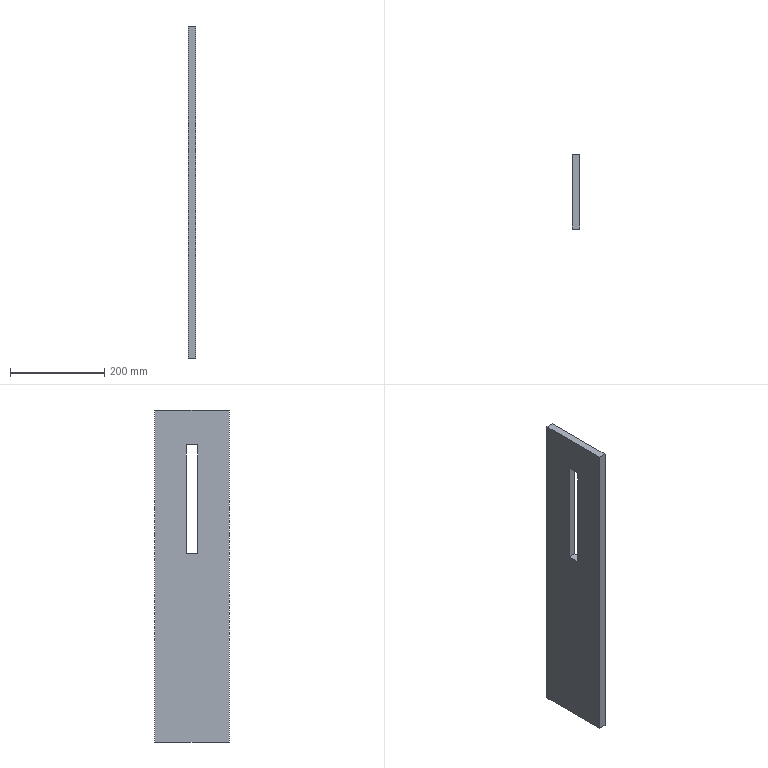Part | STEP file | 05-Vertical plate 1 | 1 solid | 10 faces | box 16 x 158 x 703 mm | volume 1685184 mm3 | plane 10
STEP:
#1=CARTESIAN_POINT('',(0.,0.,0.));
#2=DIRECTION('',(0.,0.,1.));
#3=DIRECTION('',(1.,0.,0.));
#4=AXIS2_PLACEMENT_3D('',#1,#2,#3);
#5=CARTESIAN_POINT('',(0.,-91.5,629.));
#6=VERTEX_POINT('',#5);
#7=CARTESIAN_POINT('',(0.,-66.5,629.));
#8=VERTEX_POINT('',#7);
#9=CARTESIAN_POINT('',(0.,-91.5,629.));
#10=DIRECTION('',(0.,1.,0.));
#11=VECTOR('',#10,1.);
#12=LINE('',#9,#11);
#13=CARTESIAN_POINT('',(0.,0.,703.));
#14=DIRECTION('',(1.,0.,0.));
#15=DIRECTION('',(0.,1.,0.));
#16=AXIS2_PLACEMENT_3D('',#13,#14,#15);
#17=PLANE('',#16);
#18=CARTESIAN_POINT('',(-91.5,-74.));
#19=DIRECTION('',(1.,0.));
#20=VECTOR('',#19,1.);
#21=LINE('',#18,#20);
#22=(GEOMETRIC_REPRESENTATION_CONTEXT(2)PARAMETRIC_REPRESENTATION_CONTEXT()REPRESENTATION_CONTEXT('',''));
#23=DEFINITIONAL_REPRESENTATION('',(#21),#22);
#24=PCURVE('',#17,#23);
#25=CARTESIAN_POINT('',(342.,-91.5,629.));
#26=DIRECTION('',(0.,0.,1.));
#27=DIRECTION('',(0.,-1.,0.));
#28=AXIS2_PLACEMENT_3D('',#25,#26,#27);
#29=PLANE('',#28);
#30=CARTESIAN_POINT('',(0.,-342.));
#31=DIRECTION('',(-1.,0.));
#32=VECTOR('',#31,1.);
#33=LINE('',#30,#32);
#34=(GEOMETRIC_REPRESENTATION_CONTEXT(2)PARAMETRIC_REPRESENTATION_CONTEXT()REPRESENTATION_CONTEXT('',''));
#35=DEFINITIONAL_REPRESENTATION('',(#33),#34);
#36=PCURVE('',#29,#35);
#37=SURFACE_CURVE('',#12,(#24,#36),.PCURVE_S1.);
#38=EDGE_CURVE('',#6,#8,#37,.T.);
#39=ORIENTED_EDGE('',*,*,#38,.F.);
#40=CARTESIAN_POINT('',(0.,-91.5,399.));
#41=VERTEX_POINT('',#40);
#42=CARTESIAN_POINT('',(0.,-91.5,399.));
#43=DIRECTION('',(0.,0.,1.));
#44=VECTOR('',#43,1.);
#45=LINE('',#42,#44);
#46=CARTESIAN_POINT('',(-91.5,-304.));
#47=DIRECTION('',(0.,1.));
#48=VECTOR('',#47,1.);
#49=LINE('',#46,#48);
#50=(GEOMETRIC_REPRESENTATION_CONTEXT(2)PARAMETRIC_REPRESENTATION_CONTEXT()REPRESENTATION_CONTEXT('',''));
#51=DEFINITIONAL_REPRESENTATION('',(#49),#50);
#52=PCURVE('',#17,#51);
#53=CARTESIAN_POINT('',(342.,-91.5,399.));
#54=DIRECTION('',(0.,-1.,0.));
#55=DIRECTION('',(-1.,0.,0.));
#56=AXIS2_PLACEMENT_3D('',#53,#54,#55);
#57=PLANE('',#56);
#58=CARTESIAN_POINT('',(342.,0.));
#59=DIRECTION('',(0.,-1.));
#60=VECTOR('',#59,1.);
#61=LINE('',#58,#60);
#62=(GEOMETRIC_REPRESENTATION_CONTEXT(2)PARAMETRIC_REPRESENTATION_CONTEXT()REPRESENTATION_CONTEXT('',''));
#63=DEFINITIONAL_REPRESENTATION('',(#61),#62);
#64=PCURVE('',#57,#63);
#65=SURFACE_CURVE('',#45,(#52,#64),.PCURVE_S1.);
#66=EDGE_CURVE('',#41,#6,#65,.T.);
#67=ORIENTED_EDGE('',*,*,#66,.F.);
#68=CARTESIAN_POINT('',(0.,-66.5,399.));
#69=VERTEX_POINT('',#68);
#70=CARTESIAN_POINT('',(0.,-91.5,399.));
#71=DIRECTION('',(0.,-1.,0.));
#72=VECTOR('',#71,1.);
#73=LINE('',#70,#72);
#74=CARTESIAN_POINT('',(-91.5,-304.));
#75=DIRECTION('',(-1.,0.));
#76=VECTOR('',#75,1.);
#77=LINE('',#74,#76);
#78=(GEOMETRIC_REPRESENTATION_CONTEXT(2)PARAMETRIC_REPRESENTATION_CONTEXT()REPRESENTATION_CONTEXT('',''));
#79=DEFINITIONAL_REPRESENTATION('',(#77),#78);
#80=PCURVE('',#17,#79);
#81=CARTESIAN_POINT('',(342.,-91.5,399.));
#82=DIRECTION('',(0.,0.,-1.));
#83=DIRECTION('',(0.,1.,0.));
#84=AXIS2_PLACEMENT_3D('',#81,#82,#83);
#85=PLANE('',#84);
#86=CARTESIAN_POINT('',(0.,-342.));
#87=DIRECTION('',(-1.,0.));
#88=VECTOR('',#87,1.);
#89=LINE('',#86,#88);
#90=(GEOMETRIC_REPRESENTATION_CONTEXT(2)PARAMETRIC_REPRESENTATION_CONTEXT()REPRESENTATION_CONTEXT('',''));
#91=DEFINITIONAL_REPRESENTATION('',(#89),#90);
#92=PCURVE('',#85,#91);
#93=SURFACE_CURVE('',#73,(#80,#92),.PCURVE_S1.);
#94=EDGE_CURVE('',#69,#41,#93,.T.);
#95=ORIENTED_EDGE('',*,*,#94,.F.);
#96=CARTESIAN_POINT('',(0.,-66.5,399.));
#97=DIRECTION('',(0.,0.,-1.));
#98=VECTOR('',#97,1.);
#99=LINE('',#96,#98);
#100=CARTESIAN_POINT('',(-66.5,-304.));
#101=DIRECTION('',(0.,-1.));
#102=VECTOR('',#101,1.);
#103=LINE('',#100,#102);
#104=(GEOMETRIC_REPRESENTATION_CONTEXT(2)PARAMETRIC_REPRESENTATION_CONTEXT()REPRESENTATION_CONTEXT('',''));
#105=DEFINITIONAL_REPRESENTATION('',(#103),#104);
#106=PCURVE('',#17,#105);
#107=CARTESIAN_POINT('',(342.,-66.5,399.));
#108=DIRECTION('',(0.,1.,0.));
#109=DIRECTION('',(1.,0.,0.));
#110=AXIS2_PLACEMENT_3D('',#107,#108,#109);
#111=PLANE('',#110);
#112=CARTESIAN_POINT('',(-342.,0.));
#113=DIRECTION('',(0.,1.));
#114=VECTOR('',#113,1.);
#115=LINE('',#112,#114);
#116=(GEOMETRIC_REPRESENTATION_CONTEXT(2)PARAMETRIC_REPRESENTATION_CONTEXT()REPRESENTATION_CONTEXT('',''));
#117=DEFINITIONAL_REPRESENTATION('',(#115),#116);
#118=PCURVE('',#111,#117);
#119=SURFACE_CURVE('',#99,(#106,#118),.PCURVE_S1.);
#120=EDGE_CURVE('',#8,#69,#119,.T.);
#121=ORIENTED_EDGE('',*,*,#120,.F.);
#122=EDGE_LOOP('',(#39,#67,#95,#121));
#123=FACE_BOUND('',#122,.T.);
#124=CARTESIAN_POINT('',(0.,0.,0.));
#125=VERTEX_POINT('',#124);
#126=CARTESIAN_POINT('',(0.,-158.,0.));
#127=VERTEX_POINT('',#126);
#128=CARTESIAN_POINT('',(0.,0.,0.));
#129=DIRECTION('',(0.,-1.,0.));
#130=VECTOR('',#129,1.);
#131=LINE('',#128,#130);
#132=CARTESIAN_POINT('',(0.,-703.));
#133=DIRECTION('',(-1.,0.));
#134=VECTOR('',#133,1.);
#135=LINE('',#132,#134);
#136=(GEOMETRIC_REPRESENTATION_CONTEXT(2)PARAMETRIC_REPRESENTATION_CONTEXT()REPRESENTATION_CONTEXT('',''));
#137=DEFINITIONAL_REPRESENTATION('',(#135),#136);
#138=PCURVE('',#17,#137);
#139=CARTESIAN_POINT('',(0.,0.,0.));
#140=DIRECTION('',(0.,0.,1.));
#141=DIRECTION('',(1.,0.,0.));
#142=AXIS2_PLACEMENT_3D('',#139,#140,#141);
#143=PLANE('',#142);
#144=CARTESIAN_POINT('',(0.,0.));
#145=DIRECTION('',(0.,-1.));
#146=VECTOR('',#145,1.);
#147=LINE('',#144,#146);
#148=(GEOMETRIC_REPRESENTATION_CONTEXT(2)PARAMETRIC_REPRESENTATION_CONTEXT()REPRESENTATION_CONTEXT('',''));
#149=DEFINITIONAL_REPRESENTATION('',(#147),#148);
#150=PCURVE('',#143,#149);
#151=SURFACE_CURVE('',#131,(#138,#150),.PCURVE_S1.);
#152=EDGE_CURVE('',#125,#127,#151,.T.);
#153=ORIENTED_EDGE('',*,*,#152,.T.);
#154=CARTESIAN_POINT('',(0.,-158.,703.));
#155=VERTEX_POINT('',#154);
#156=CARTESIAN_POINT('',(0.,-158.,703.));
#157=DIRECTION('',(0.,0.,-1.));
#158=VECTOR('',#157,1.);
#159=LINE('',#156,#158);
#160=CARTESIAN_POINT('',(-158.,0.));
#161=DIRECTION('',(0.,-1.));
#162=VECTOR('',#161,1.);
#163=LINE('',#160,#162);
#164=(GEOMETRIC_REPRESENTATION_CONTEXT(2)PARAMETRIC_REPRESENTATION_CONTEXT()REPRESENTATION_CONTEXT('',''));
#165=DEFINITIONAL_REPRESENTATION('',(#163),#164);
#166=PCURVE('',#17,#165);
#167=CARTESIAN_POINT('',(0.,-158.,703.));
#168=DIRECTION('',(0.,1.,0.));
#169=DIRECTION('',(0.,0.,1.));
#170=AXIS2_PLACEMENT_3D('',#167,#168,#169);
#171=PLANE('',#170);
#172=CARTESIAN_POINT('',(0.,0.));
#173=DIRECTION('',(-1.,0.));
#174=VECTOR('',#173,1.);
#175=LINE('',#172,#174);
#176=(GEOMETRIC_REPRESENTATION_CONTEXT(2)PARAMETRIC_REPRESENTATION_CONTEXT()REPRESENTATION_CONTEXT('',''));
#177=DEFINITIONAL_REPRESENTATION('',(#175),#176);
#178=PCURVE('',#171,#177);
#179=SURFACE_CURVE('',#159,(#166,#178),.PCURVE_S1.);
#180=EDGE_CURVE('',#155,#127,#179,.T.);
#181=ORIENTED_EDGE('',*,*,#180,.F.);
#182=CARTESIAN_POINT('',(0.,0.,703.));
#183=VERTEX_POINT('',#182);
#184=CARTESIAN_POINT('',(0.,0.,703.));
#185=DIRECTION('',(0.,-1.,0.));
#186=VECTOR('',#185,1.);
#187=LINE('',#184,#186);
#188=CARTESIAN_POINT('',(0.,0.));
#189=DIRECTION('',(-1.,0.));
#190=VECTOR('',#189,1.);
#191=LINE('',#188,#190);
#192=(GEOMETRIC_REPRESENTATION_CONTEXT(2)PARAMETRIC_REPRESENTATION_CONTEXT()REPRESENTATION_CONTEXT('',''));
#193=DEFINITIONAL_REPRESENTATION('',(#191),#192);
#194=PCURVE('',#17,#193);
#195=CARTESIAN_POINT('',(0.,0.,703.));
#196=DIRECTION('',(0.,0.,1.));
#197=DIRECTION('',(1.,0.,0.));
#198=AXIS2_PLACEMENT_3D('',#195,#196,#197);
#199=PLANE('',#198);
#200=CARTESIAN_POINT('',(0.,0.));
#201=DIRECTION('',(0.,-1.));
#202=VECTOR('',#201,1.);
#203=LINE('',#200,#202);
#204=(GEOMETRIC_REPRESENTATION_CONTEXT(2)PARAMETRIC_REPRESENTATION_CONTEXT()REPRESENTATION_CONTEXT('',''));
#205=DEFINITIONAL_REPRESENTATION('',(#203),#204);
#206=PCURVE('',#199,#205);
#207=SURFACE_CURVE('',#187,(#194,#206),.PCURVE_S1.);
#208=EDGE_CURVE('',#183,#155,#207,.T.);
#209=ORIENTED_EDGE('',*,*,#208,.F.);
#210=CARTESIAN_POINT('',(0.,0.,703.));
#211=DIRECTION('',(0.,0.,-1.));
#212=VECTOR('',#211,1.);
#213=LINE('',#210,#212);
#214=CARTESIAN_POINT('',(0.,0.));
#215=DIRECTION('',(0.,-1.));
#216=VECTOR('',#215,1.);
#217=LINE('',#214,#216);
#218=(GEOMETRIC_REPRESENTATION_CONTEXT(2)PARAMETRIC_REPRESENTATION_CONTEXT()REPRESENTATION_CONTEXT('',''));
#219=DEFINITIONAL_REPRESENTATION('',(#217),#218);
#220=PCURVE('',#17,#219);
#221=CARTESIAN_POINT('',(0.,0.,703.));
#222=DIRECTION('',(0.,-1.,0.));
#223=DIRECTION('',(0.,0.,-1.));
#224=AXIS2_PLACEMENT_3D('',#221,#222,#223);
#225=PLANE('',#224);
#226=CARTESIAN_POINT('',(0.,0.));
#227=DIRECTION('',(1.,0.));
#228=VECTOR('',#227,1.);
#229=LINE('',#226,#228);
#230=(GEOMETRIC_REPRESENTATION_CONTEXT(2)PARAMETRIC_REPRESENTATION_CONTEXT()REPRESENTATION_CONTEXT('',''));
#231=DEFINITIONAL_REPRESENTATION('',(#229),#230);
#232=PCURVE('',#225,#231);
#233=SURFACE_CURVE('',#213,(#220,#232),.PCURVE_S1.);
#234=EDGE_CURVE('',#183,#125,#233,.T.);
#235=ORIENTED_EDGE('',*,*,#234,.T.);
#236=EDGE_LOOP('',(#153,#181,#209,#235));
#237=FACE_BOUND('',#236,.T.);
#238=ADVANCED_FACE('',(#123,#237),#17,.F.);
#239=CARTESIAN_POINT('',(16.,-158.,0.));
#240=VERTEX_POINT('',#239);
#241=CARTESIAN_POINT('',(0.,-158.,0.));
#242=DIRECTION('',(1.,0.,0.));
#243=VECTOR('',#242,1.);
#244=LINE('',#241,#243);
#245=CARTESIAN_POINT('',(-703.,0.));
#246=DIRECTION('',(0.,1.));
#247=VECTOR('',#246,1.);
#248=LINE('',#245,#247);
#249=(GEOMETRIC_REPRESENTATION_CONTEXT(2)PARAMETRIC_REPRESENTATION_CONTEXT()REPRESENTATION_CONTEXT('',''));
#250=DEFINITIONAL_REPRESENTATION('',(#248),#249);
#251=PCURVE('',#171,#250);
#252=CARTESIAN_POINT('',(0.,-158.));
#253=DIRECTION('',(1.,0.));
#254=VECTOR('',#253,1.);
#255=LINE('',#252,#254);
#256=(GEOMETRIC_REPRESENTATION_CONTEXT(2)PARAMETRIC_REPRESENTATION_CONTEXT()REPRESENTATION_CONTEXT('',''));
#257=DEFINITIONAL_REPRESENTATION('',(#255),#256);
#258=PCURVE('',#143,#257);
#259=SURFACE_CURVE('',#244,(#251,#258),.PCURVE_S1.);
#260=EDGE_CURVE('',#127,#240,#259,.T.);
#261=ORIENTED_EDGE('',*,*,#260,.T.);
#262=CARTESIAN_POINT('',(16.,-158.,703.));
#263=VERTEX_POINT('',#262);
#264=CARTESIAN_POINT('',(16.,-158.,703.));
#265=DIRECTION('',(0.,0.,-1.));
#266=VECTOR('',#265,1.);
#267=LINE('',#264,#266);
#268=CARTESIAN_POINT('',(0.,16.));
#269=DIRECTION('',(-1.,0.));
#270=VECTOR('',#269,1.);
#271=LINE('',#268,#270);
#272=(GEOMETRIC_REPRESENTATION_CONTEXT(2)PARAMETRIC_REPRESENTATION_CONTEXT()REPRESENTATION_CONTEXT('',''));
#273=DEFINITIONAL_REPRESENTATION('',(#271),#272);
#274=PCURVE('',#171,#273);
#275=CARTESIAN_POINT('',(16.,0.,703.));
#276=DIRECTION('',(-1.,0.,0.));
#277=DIRECTION('',(0.,-1.,0.));
#278=AXIS2_PLACEMENT_3D('',#275,#276,#277);
#279=PLANE('',#278);
#280=CARTESIAN_POINT('',(158.,0.));
#281=DIRECTION('',(0.,-1.));
#282=VECTOR('',#281,1.);
#283=LINE('',#280,#282);
#284=(GEOMETRIC_REPRESENTATION_CONTEXT(2)PARAMETRIC_REPRESENTATION_CONTEXT()REPRESENTATION_CONTEXT('',''));
#285=DEFINITIONAL_REPRESENTATION('',(#283),#284);
#286=PCURVE('',#279,#285);
#287=SURFACE_CURVE('',#267,(#274,#286),.PCURVE_S1.);
#288=EDGE_CURVE('',#263,#240,#287,.T.);
#289=ORIENTED_EDGE('',*,*,#288,.F.);
#290=CARTESIAN_POINT('',(0.,-158.,703.));
#291=DIRECTION('',(1.,0.,0.));
#292=VECTOR('',#291,1.);
#293=LINE('',#290,#292);
#294=CARTESIAN_POINT('',(0.,0.));
#295=DIRECTION('',(0.,1.));
#296=VECTOR('',#295,1.);
#297=LINE('',#294,#296);
#298=(GEOMETRIC_REPRESENTATION_CONTEXT(2)PARAMETRIC_REPRESENTATION_CONTEXT()REPRESENTATION_CONTEXT('',''));
#299=DEFINITIONAL_REPRESENTATION('',(#297),#298);
#300=PCURVE('',#171,#299);
#301=CARTESIAN_POINT('',(0.,-158.));
#302=DIRECTION('',(1.,0.));
#303=VECTOR('',#302,1.);
#304=LINE('',#301,#303);
#305=(GEOMETRIC_REPRESENTATION_CONTEXT(2)PARAMETRIC_REPRESENTATION_CONTEXT()REPRESENTATION_CONTEXT('',''));
#306=DEFINITIONAL_REPRESENTATION('',(#304),#305);
#307=PCURVE('',#199,#306);
#308=SURFACE_CURVE('',#293,(#300,#307),.PCURVE_S1.);
#309=EDGE_CURVE('',#155,#263,#308,.T.);
#310=ORIENTED_EDGE('',*,*,#309,.F.);
#311=ORIENTED_EDGE('',*,*,#180,.T.);
#312=EDGE_LOOP('',(#261,#289,#310,#311));
#313=FACE_BOUND('',#312,.T.);
#314=ADVANCED_FACE('',(#313),#171,.F.);
#315=CARTESIAN_POINT('',(16.,-66.5,399.));
#316=VERTEX_POINT('',#315);
#317=CARTESIAN_POINT('',(16.,-91.5,399.));
#318=VERTEX_POINT('',#317);
#319=CARTESIAN_POINT('',(16.,0.,399.));
#320=DIRECTION('',(0.,-1.,0.));
#321=VECTOR('',#320,1.);
#322=LINE('',#319,#321);
#323=CARTESIAN_POINT('',(0.,-304.));
#324=DIRECTION('',(1.,0.));
#325=VECTOR('',#324,1.);
#326=LINE('',#323,#325);
#327=(GEOMETRIC_REPRESENTATION_CONTEXT(2)PARAMETRIC_REPRESENTATION_CONTEXT()REPRESENTATION_CONTEXT('',''));
#328=DEFINITIONAL_REPRESENTATION('',(#326),#327);
#329=PCURVE('',#279,#328);
#330=CARTESIAN_POINT('',(91.5,-326.));
#331=DIRECTION('',(-1.,0.));
#332=VECTOR('',#331,1.);
#333=LINE('',#330,#332);
#334=(GEOMETRIC_REPRESENTATION_CONTEXT(2)PARAMETRIC_REPRESENTATION_CONTEXT()REPRESENTATION_CONTEXT('',''));
#335=DEFINITIONAL_REPRESENTATION('',(#333),#334);
#336=PCURVE('',#85,#335);
#337=SURFACE_CURVE('',#322,(#329,#336),.PCURVE_S1.);
#338=EDGE_CURVE('',#316,#318,#337,.T.);
#339=ORIENTED_EDGE('',*,*,#338,.T.);
#340=CARTESIAN_POINT('',(16.,-91.5,629.));
#341=VERTEX_POINT('',#340);
#342=CARTESIAN_POINT('',(16.,-91.5,703.));
#343=DIRECTION('',(0.,0.,1.));
#344=VECTOR('',#343,1.);
#345=LINE('',#342,#344);
#346=CARTESIAN_POINT('',(91.5,0.));
#347=DIRECTION('',(0.,1.));
#348=VECTOR('',#347,1.);
#349=LINE('',#346,#348);
#350=(GEOMETRIC_REPRESENTATION_CONTEXT(2)PARAMETRIC_REPRESENTATION_CONTEXT()REPRESENTATION_CONTEXT('',''));
#351=DEFINITIONAL_REPRESENTATION('',(#349),#350);
#352=PCURVE('',#279,#351);
#353=CARTESIAN_POINT('',(326.,-304.));
#354=DIRECTION('',(0.,-1.));
#355=VECTOR('',#354,1.);
#356=LINE('',#353,#355);
#357=(GEOMETRIC_REPRESENTATION_CONTEXT(2)PARAMETRIC_REPRESENTATION_CONTEXT()REPRESENTATION_CONTEXT('',''));
#358=DEFINITIONAL_REPRESENTATION('',(#356),#357);
#359=PCURVE('',#57,#358);
#360=SURFACE_CURVE('',#345,(#352,#359),.PCURVE_S1.);
#361=EDGE_CURVE('',#318,#341,#360,.T.);
#362=ORIENTED_EDGE('',*,*,#361,.T.);
#363=CARTESIAN_POINT('',(16.,-66.5,629.));
#364=VERTEX_POINT('',#363);
#365=CARTESIAN_POINT('',(16.,0.,629.));
#366=DIRECTION('',(0.,1.,0.));
#367=VECTOR('',#366,1.);
#368=LINE('',#365,#367);
#369=CARTESIAN_POINT('',(0.,-74.));
#370=DIRECTION('',(-1.,0.));
#371=VECTOR('',#370,1.);
#372=LINE('',#369,#371);
#373=(GEOMETRIC_REPRESENTATION_CONTEXT(2)PARAMETRIC_REPRESENTATION_CONTEXT()REPRESENTATION_CONTEXT('',''));
#374=DEFINITIONAL_REPRESENTATION('',(#372),#373);
#375=PCURVE('',#279,#374);
#376=CARTESIAN_POINT('',(-91.5,-326.));
#377=DIRECTION('',(-1.,0.));
#378=VECTOR('',#377,1.);
#379=LINE('',#376,#378);
#380=(GEOMETRIC_REPRESENTATION_CONTEXT(2)PARAMETRIC_REPRESENTATION_CONTEXT()REPRESENTATION_CONTEXT('',''));
#381=DEFINITIONAL_REPRESENTATION('',(#379),#380);
#382=PCURVE('',#29,#381);
#383=SURFACE_CURVE('',#368,(#375,#382),.PCURVE_S1.);
#384=EDGE_CURVE('',#341,#364,#383,.T.);
#385=ORIENTED_EDGE('',*,*,#384,.T.);
#386=CARTESIAN_POINT('',(16.,-66.5,703.));
#387=DIRECTION('',(0.,0.,-1.));
#388=VECTOR('',#387,1.);
#389=LINE('',#386,#388);
#390=CARTESIAN_POINT('',(66.5,0.));
#391=DIRECTION('',(0.,-1.));
#392=VECTOR('',#391,1.);
#393=LINE('',#390,#392);
#394=(GEOMETRIC_REPRESENTATION_CONTEXT(2)PARAMETRIC_REPRESENTATION_CONTEXT()REPRESENTATION_CONTEXT('',''));
#395=DEFINITIONAL_REPRESENTATION('',(#393),#394);
#396=PCURVE('',#279,#395);
#397=CARTESIAN_POINT('',(-326.,-304.));
#398=DIRECTION('',(0.,1.));
#399=VECTOR('',#398,1.);
#400=LINE('',#397,#399);
#401=(GEOMETRIC_REPRESENTATION_CONTEXT(2)PARAMETRIC_REPRESENTATION_CONTEXT()REPRESENTATION_CONTEXT('',''));
#402=DEFINITIONAL_REPRESENTATION('',(#400),#401);
#403=PCURVE('',#111,#402);
#404=SURFACE_CURVE('',#389,(#396,#403),.PCURVE_S1.);
#405=EDGE_CURVE('',#364,#316,#404,.T.);
#406=ORIENTED_EDGE('',*,*,#405,.T.);
#407=EDGE_LOOP('',(#339,#362,#385,#406));
#408=FACE_BOUND('',#407,.T.);
#409=CARTESIAN_POINT('',(16.,0.,0.));
#410=VERTEX_POINT('',#409);
#411=CARTESIAN_POINT('',(16.,0.,0.));
#412=DIRECTION('',(0.,1.,0.));
#413=VECTOR('',#412,1.);
#414=LINE('',#411,#413);
#415=CARTESIAN_POINT('',(0.,-703.));
#416=DIRECTION('',(-1.,0.));
#417=VECTOR('',#416,1.);
#418=LINE('',#415,#417);
#419=(GEOMETRIC_REPRESENTATION_CONTEXT(2)PARAMETRIC_REPRESENTATION_CONTEXT()REPRESENTATION_CONTEXT('',''));
#420=DEFINITIONAL_REPRESENTATION('',(#418),#419);
#421=PCURVE('',#279,#420);
#422=CARTESIAN_POINT('',(16.,0.));
#423=DIRECTION('',(0.,1.));
#424=VECTOR('',#423,1.);
#425=LINE('',#422,#424);
#426=(GEOMETRIC_REPRESENTATION_CONTEXT(2)PARAMETRIC_REPRESENTATION_CONTEXT()REPRESENTATION_CONTEXT('',''));
#427=DEFINITIONAL_REPRESENTATION('',(#425),#426);
#428=PCURVE('',#143,#427);
#429=SURFACE_CURVE('',#414,(#421,#428),.PCURVE_S1.);
#430=EDGE_CURVE('',#240,#410,#429,.T.);
#431=ORIENTED_EDGE('',*,*,#430,.T.);
#432=CARTESIAN_POINT('',(16.,0.,703.));
#433=VERTEX_POINT('',#432);
#434=CARTESIAN_POINT('',(16.,0.,703.));
#435=DIRECTION('',(0.,0.,-1.));
#436=VECTOR('',#435,1.);
#437=LINE('',#434,#436);
#438=CARTESIAN_POINT('',(0.,0.));
#439=DIRECTION('',(0.,-1.));
#440=VECTOR('',#439,1.);
#441=LINE('',#438,#440);
#442=(GEOMETRIC_REPRESENTATION_CONTEXT(2)PARAMETRIC_REPRESENTATION_CONTEXT()REPRESENTATION_CONTEXT('',''));
#443=DEFINITIONAL_REPRESENTATION('',(#441),#442);
#444=PCURVE('',#279,#443);
#445=CARTESIAN_POINT('',(0.,16.));
#446=DIRECTION('',(1.,0.));
#447=VECTOR('',#446,1.);
#448=LINE('',#445,#447);
#449=(GEOMETRIC_REPRESENTATION_CONTEXT(2)PARAMETRIC_REPRESENTATION_CONTEXT()REPRESENTATION_CONTEXT('',''));
#450=DEFINITIONAL_REPRESENTATION('',(#448),#449);
#451=PCURVE('',#225,#450);
#452=SURFACE_CURVE('',#437,(#444,#451),.PCURVE_S1.);
#453=EDGE_CURVE('',#433,#410,#452,.T.);
#454=ORIENTED_EDGE('',*,*,#453,.F.);
#455=CARTESIAN_POINT('',(16.,0.,703.));
#456=DIRECTION('',(0.,1.,0.));
#457=VECTOR('',#456,1.);
#458=LINE('',#455,#457);
#459=CARTESIAN_POINT('',(0.,0.));
#460=DIRECTION('',(-1.,0.));
#461=VECTOR('',#460,1.);
#462=LINE('',#459,#461);
#463=(GEOMETRIC_REPRESENTATION_CONTEXT(2)PARAMETRIC_REPRESENTATION_CONTEXT()REPRESENTATION_CONTEXT('',''));
#464=DEFINITIONAL_REPRESENTATION('',(#462),#463);
#465=PCURVE('',#279,#464);
#466=CARTESIAN_POINT('',(16.,0.));
#467=DIRECTION('',(0.,1.));
#468=VECTOR('',#467,1.);
#469=LINE('',#466,#468);
#470=(GEOMETRIC_REPRESENTATION_CONTEXT(2)PARAMETRIC_REPRESENTATION_CONTEXT()REPRESENTATION_CONTEXT('',''));
#471=DEFINITIONAL_REPRESENTATION('',(#469),#470);
#472=PCURVE('',#199,#471);
#473=SURFACE_CURVE('',#458,(#465,#472),.PCURVE_S1.);
#474=EDGE_CURVE('',#263,#433,#473,.T.);
#475=ORIENTED_EDGE('',*,*,#474,.F.);
#476=ORIENTED_EDGE('',*,*,#288,.T.);
#477=EDGE_LOOP('',(#431,#454,#475,#476));
#478=FACE_BOUND('',#477,.T.);
#479=ADVANCED_FACE('',(#408,#478),#279,.F.);
#480=CARTESIAN_POINT('',(0.,0.,0.));
#481=DIRECTION('',(-1.,0.,0.));
#482=VECTOR('',#481,1.);
#483=LINE('',#480,#482);
#484=CARTESIAN_POINT('',(703.,0.));
#485=DIRECTION('',(0.,-1.));
#486=VECTOR('',#485,1.);
#487=LINE('',#484,#486);
#488=(GEOMETRIC_REPRESENTATION_CONTEXT(2)PARAMETRIC_REPRESENTATION_CONTEXT()REPRESENTATION_CONTEXT('',''));
#489=DEFINITIONAL_REPRESENTATION('',(#487),#488);
#490=PCURVE('',#225,#489);
#491=CARTESIAN_POINT('',(0.,0.));
#492=DIRECTION('',(-1.,0.));
#493=VECTOR('',#492,1.);
#494=LINE('',#491,#493);
#495=(GEOMETRIC_REPRESENTATION_CONTEXT(2)PARAMETRIC_REPRESENTATION_CONTEXT()REPRESENTATION_CONTEXT('',''));
#496=DEFINITIONAL_REPRESENTATION('',(#494),#495);
#497=PCURVE('',#143,#496);
#498=SURFACE_CURVE('',#483,(#490,#497),.PCURVE_S1.);
#499=EDGE_CURVE('',#410,#125,#498,.T.);
#500=ORIENTED_EDGE('',*,*,#499,.T.);
#501=ORIENTED_EDGE('',*,*,#234,.F.);
#502=CARTESIAN_POINT('',(0.,0.,703.));
#503=DIRECTION('',(-1.,0.,0.));
#504=VECTOR('',#503,1.);
#505=LINE('',#502,#504);
#506=CARTESIAN_POINT('',(0.,0.));
#507=DIRECTION('',(0.,-1.));
#508=VECTOR('',#507,1.);
#509=LINE('',#506,#508);
#510=(GEOMETRIC_REPRESENTATION_CONTEXT(2)PARAMETRIC_REPRESENTATION_CONTEXT()REPRESENTATION_CONTEXT('',''));
#511=DEFINITIONAL_REPRESENTATION('',(#509),#510);
#512=PCURVE('',#225,#511);
#513=CARTESIAN_POINT('',(0.,0.));
#514=DIRECTION('',(-1.,0.));
#515=VECTOR('',#514,1.);
#516=LINE('',#513,#515);
#517=(GEOMETRIC_REPRESENTATION_CONTEXT(2)PARAMETRIC_REPRESENTATION_CONTEXT()REPRESENTATION_CONTEXT('',''));
#518=DEFINITIONAL_REPRESENTATION('',(#516),#517);
#519=PCURVE('',#199,#518);
#520=SURFACE_CURVE('',#505,(#512,#519),.PCURVE_S1.);
#521=EDGE_CURVE('',#433,#183,#520,.T.);
#522=ORIENTED_EDGE('',*,*,#521,.F.);
#523=ORIENTED_EDGE('',*,*,#453,.T.);
#524=EDGE_LOOP('',(#500,#501,#522,#523));
#525=FACE_BOUND('',#524,.T.);
#526=ADVANCED_FACE('',(#525),#225,.F.);
#527=ORIENTED_EDGE('',*,*,#208,.T.);
#528=ORIENTED_EDGE('',*,*,#309,.T.);
#529=ORIENTED_EDGE('',*,*,#474,.T.);
#530=ORIENTED_EDGE('',*,*,#521,.T.);
#531=EDGE_LOOP('',(#527,#528,#529,#530));
#532=FACE_BOUND('',#531,.T.);
#533=ADVANCED_FACE('',(#532),#199,.T.);
#534=ORIENTED_EDGE('',*,*,#152,.F.);
#535=ORIENTED_EDGE('',*,*,#499,.F.);
#536=ORIENTED_EDGE('',*,*,#430,.F.);
#537=ORIENTED_EDGE('',*,*,#260,.F.);
#538=EDGE_LOOP('',(#534,#535,#536,#537));
#539=FACE_BOUND('',#538,.T.);
#540=ADVANCED_FACE('',(#539),#143,.F.);
#541=CARTESIAN_POINT('',(342.,-91.5,399.));
#542=DIRECTION('',(-1.,0.,0.));
#543=VECTOR('',#542,1.);
#544=LINE('',#541,#543);
#545=CARTESIAN_POINT('',(0.,0.));
#546=DIRECTION('',(1.,0.));
#547=VECTOR('',#546,1.);
#548=LINE('',#545,#547);
#549=(GEOMETRIC_REPRESENTATION_CONTEXT(2)PARAMETRIC_REPRESENTATION_CONTEXT()REPRESENTATION_CONTEXT('',''));
#550=DEFINITIONAL_REPRESENTATION('',(#548),#549);
#551=PCURVE('',#57,#550);
#552=CARTESIAN_POINT('',(0.,0.));
#553=DIRECTION('',(0.,-1.));
#554=VECTOR('',#553,1.);
#555=LINE('',#552,#554);
#556=(GEOMETRIC_REPRESENTATION_CONTEXT(2)PARAMETRIC_REPRESENTATION_CONTEXT()REPRESENTATION_CONTEXT('',''));
#557=DEFINITIONAL_REPRESENTATION('',(#555),#556);
#558=PCURVE('',#85,#557);
#559=SURFACE_CURVE('',#544,(#551,#558),.PCURVE_S1.);
#560=EDGE_CURVE('',#318,#41,#559,.T.);
#561=ORIENTED_EDGE('',*,*,#560,.T.);
#562=ORIENTED_EDGE('',*,*,#66,.T.);
#563=CARTESIAN_POINT('',(342.,-91.5,629.));
#564=DIRECTION('',(-1.,0.,0.));
#565=VECTOR('',#564,1.);
#566=LINE('',#563,#565);
#567=CARTESIAN_POINT('',(0.,-230.));
#568=DIRECTION('',(1.,0.));
#569=VECTOR('',#568,1.);
#570=LINE('',#567,#569);
#571=(GEOMETRIC_REPRESENTATION_CONTEXT(2)PARAMETRIC_REPRESENTATION_CONTEXT()REPRESENTATION_CONTEXT('',''));
#572=DEFINITIONAL_REPRESENTATION('',(#570),#571);
#573=PCURVE('',#57,#572);
#574=CARTESIAN_POINT('',(0.,0.));
#575=DIRECTION('',(0.,-1.));
#576=VECTOR('',#575,1.);
#577=LINE('',#574,#576);
#578=(GEOMETRIC_REPRESENTATION_CONTEXT(2)PARAMETRIC_REPRESENTATION_CONTEXT()REPRESENTATION_CONTEXT('',''));
#579=DEFINITIONAL_REPRESENTATION('',(#577),#578);
#580=PCURVE('',#29,#579);
#581=SURFACE_CURVE('',#566,(#573,#580),.PCURVE_S1.);
#582=EDGE_CURVE('',#341,#6,#581,.T.);
#583=ORIENTED_EDGE('',*,*,#582,.F.);
#584=ORIENTED_EDGE('',*,*,#361,.F.);
#585=EDGE_LOOP('',(#561,#562,#583,#584));
#586=FACE_BOUND('',#585,.T.);
#587=ADVANCED_FACE('',(#586),#57,.F.);
#588=CARTESIAN_POINT('',(342.,-66.5,399.));
#589=DIRECTION('',(-1.,0.,0.));
#590=VECTOR('',#589,1.);
#591=LINE('',#588,#590);
#592=CARTESIAN_POINT('',(25.,0.));
#593=DIRECTION('',(0.,-1.));
#594=VECTOR('',#593,1.);
#595=LINE('',#592,#594);
#596=(GEOMETRIC_REPRESENTATION_CONTEXT(2)PARAMETRIC_REPRESENTATION_CONTEXT()REPRESENTATION_CONTEXT('',''));
#597=DEFINITIONAL_REPRESENTATION('',(#595),#596);
#598=PCURVE('',#85,#597);
#599=CARTESIAN_POINT('',(0.,0.));
#600=DIRECTION('',(-1.,0.));
#601=VECTOR('',#600,1.);
#602=LINE('',#599,#601);
#603=(GEOMETRIC_REPRESENTATION_CONTEXT(2)PARAMETRIC_REPRESENTATION_CONTEXT()REPRESENTATION_CONTEXT('',''));
#604=DEFINITIONAL_REPRESENTATION('',(#602),#603);
#605=PCURVE('',#111,#604);
#606=SURFACE_CURVE('',#591,(#598,#605),.PCURVE_S1.);
#607=EDGE_CURVE('',#316,#69,#606,.T.);
#608=ORIENTED_EDGE('',*,*,#607,.T.);
#609=ORIENTED_EDGE('',*,*,#94,.T.);
#610=ORIENTED_EDGE('',*,*,#560,.F.);
#611=ORIENTED_EDGE('',*,*,#338,.F.);
#612=EDGE_LOOP('',(#608,#609,#610,#611));
#613=FACE_BOUND('',#612,.T.);
#614=ADVANCED_FACE('',(#613),#85,.F.);
#615=CARTESIAN_POINT('',(342.,-66.5,629.));
#616=DIRECTION('',(-1.,0.,0.));
#617=VECTOR('',#616,1.);
#618=LINE('',#615,#617);
#619=CARTESIAN_POINT('',(0.,-230.));
#620=DIRECTION('',(-1.,0.));
#621=VECTOR('',#620,1.);
#622=LINE('',#619,#621);
#623=(GEOMETRIC_REPRESENTATION_CONTEXT(2)PARAMETRIC_REPRESENTATION_CONTEXT()REPRESENTATION_CONTEXT('',''));
#624=DEFINITIONAL_REPRESENTATION('',(#622),#623);
#625=PCURVE('',#111,#624);
#626=CARTESIAN_POINT('',(-25.,0.));
#627=DIRECTION('',(0.,-1.));
#628=VECTOR('',#627,1.);
#629=LINE('',#626,#628);
#630=(GEOMETRIC_REPRESENTATION_CONTEXT(2)PARAMETRIC_REPRESENTATION_CONTEXT()REPRESENTATION_CONTEXT('',''));
#631=DEFINITIONAL_REPRESENTATION('',(#629),#630);
#632=PCURVE('',#29,#631);
#633=SURFACE_CURVE('',#618,(#625,#632),.PCURVE_S1.);
#634=EDGE_CURVE('',#364,#8,#633,.T.);
#635=ORIENTED_EDGE('',*,*,#634,.T.);
#636=ORIENTED_EDGE('',*,*,#120,.T.);
#637=ORIENTED_EDGE('',*,*,#607,.F.);
#638=ORIENTED_EDGE('',*,*,#405,.F.);
#639=EDGE_LOOP('',(#635,#636,#637,#638));
#640=FACE_BOUND('',#639,.T.);
#641=ADVANCED_FACE('',(#640),#111,.F.);
#642=ORIENTED_EDGE('',*,*,#582,.T.);
#643=ORIENTED_EDGE('',*,*,#38,.T.);
#644=ORIENTED_EDGE('',*,*,#634,.F.);
#645=ORIENTED_EDGE('',*,*,#384,.F.);
#646=EDGE_LOOP('',(#642,#643,#644,#645));
#647=FACE_BOUND('',#646,.T.);
#648=ADVANCED_FACE('',(#647),#29,.F.);
#649=CLOSED_SHELL('',(#238,#314,#479,#526,#533,#540,#587,#614,#641,#648));
#650=MANIFOLD_SOLID_BREP('',#649);
#651=(LENGTH_UNIT()NAMED_UNIT(*)SI_UNIT(.MILLI.,.METRE.));
#652=UNCERTAINTY_MEASURE_WITH_UNIT(LENGTH_MEASURE(0.0000001),#651,'','');
#653=(NAMED_UNIT(*)PLANE_ANGLE_UNIT()SI_UNIT($,.RADIAN.));
#654=(NAMED_UNIT(*)SI_UNIT($,.STERADIAN.)SOLID_ANGLE_UNIT());
#655=(GEOMETRIC_REPRESENTATION_CONTEXT(3)GLOBAL_UNCERTAINTY_ASSIGNED_CONTEXT((#652))GLOBAL_UNIT_ASSIGNED_CONTEXT((#651,#653,#654))REPRESENTATION_CONTEXT('',''));
#656=ADVANCED_BREP_SHAPE_REPRESENTATION('',(#4,#650),#655);